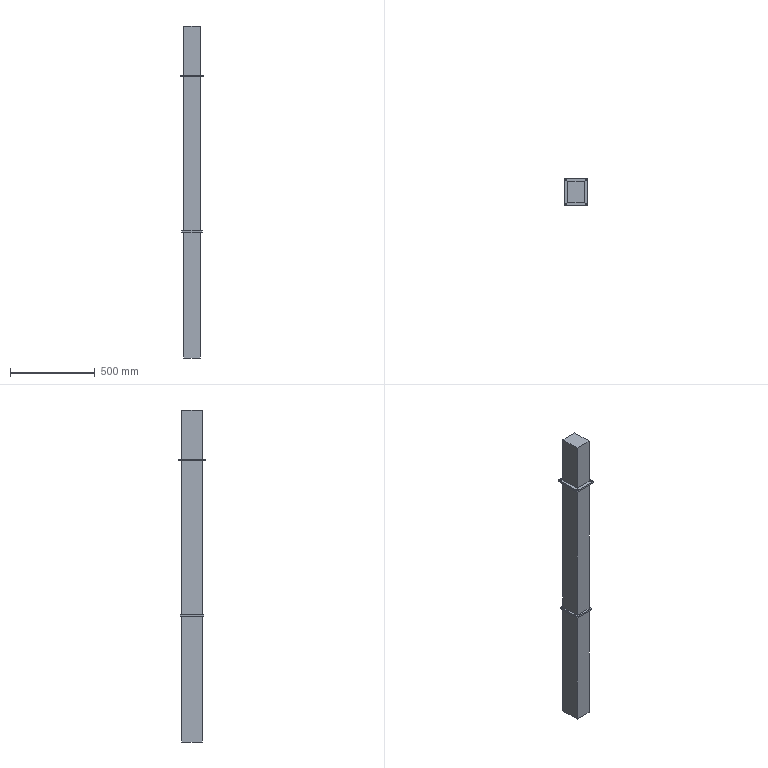Part | SolidWorks | features Cut 2, ICE 2, Extrusion 1 | 1 solid | 34 faces | box 139.912 x 160 x 1959 mm | volume 23636005 mm3 | plane 26 | cylinder 8 | commonest cylinder face diameters 10 x8
STEP:
#1=CARTESIAN_POINT('',(-54.912,230.,400.));
#2=VERTEX_POINT('',#1);
#3=CARTESIAN_POINT('',(-44.912,230.,400.));
#4=VERTEX_POINT('',#3);
#5=CARTESIAN_POINT('',(-49.912,230.,400.));
#6=DIRECTION('',(0.,0.,1.));
#7=DIRECTION('',(1.,0.,0.));
#8=AXIS2_PLACEMENT_3D('',#5,#6,#7);
#9=CIRCLE('',#8,5.);
#10=EDGE_CURVE('',#2,#4,#9,.T.);
#11=ORIENTED_EDGE('',*,*,#10,.F.);
#12=CARTESIAN_POINT('',(-54.912,230.,410.));
#13=VERTEX_POINT('',#12);
#14=CARTESIAN_POINT('',(-54.912,230.,400.));
#15=DIRECTION('',(0.,0.,1.));
#16=VECTOR('',#15,1000.);
#17=LINE('',#14,#16);
#18=EDGE_CURVE('',#2,#13,#17,.T.);
#19=ORIENTED_EDGE('',*,*,#18,.T.);
#20=CARTESIAN_POINT('',(-44.912,230.,410.));
#21=VERTEX_POINT('',#20);
#22=CARTESIAN_POINT('',(-49.912,230.,410.));
#23=DIRECTION('',(0.,0.,1.));
#24=DIRECTION('',(1.,0.,0.));
#25=AXIS2_PLACEMENT_3D('',#22,#23,#24);
#26=CIRCLE('',#25,5.);
#27=EDGE_CURVE('',#13,#21,#26,.T.);
#28=ORIENTED_EDGE('',*,*,#27,.T.);
#29=CARTESIAN_POINT('',(-44.912,230.,400.));
#30=DIRECTION('',(0.,0.,1.));
#31=VECTOR('',#30,1000.);
#32=LINE('',#29,#31);
#33=EDGE_CURVE('',#4,#21,#32,.T.);
#34=ORIENTED_EDGE('',*,*,#33,.F.);
#35=EDGE_LOOP('',(#11,#19,#28,#34));
#36=FACE_OUTER_BOUND('',#35,.T.);
#37=CARTESIAN_POINT('',(-49.912,230.,400.));
#38=DIRECTION('',(0.,0.,1.));
#39=DIRECTION('',(1.,0.,0.));
#40=AXIS2_PLACEMENT_3D('',#37,#38,#39);
#41=CYLINDRICAL_SURFACE('',#40,5.);
#42=ADVANCED_FACE('',(#36),#41,.F.);
#43=CARTESIAN_POINT('',(-54.912,90.,400.));
#44=VERTEX_POINT('',#43);
#45=CARTESIAN_POINT('',(-44.912,90.,400.));
#46=VERTEX_POINT('',#45);
#47=CARTESIAN_POINT('',(-49.912,90.,400.));
#48=DIRECTION('',(0.,0.,1.));
#49=DIRECTION('',(1.,0.,0.));
#50=AXIS2_PLACEMENT_3D('',#47,#48,#49);
#51=CIRCLE('',#50,5.);
#52=EDGE_CURVE('',#44,#46,#51,.T.);
#53=ORIENTED_EDGE('',*,*,#52,.F.);
#54=CARTESIAN_POINT('',(-54.912,90.,410.));
#55=VERTEX_POINT('',#54);
#56=CARTESIAN_POINT('',(-54.912,90.,400.));
#57=DIRECTION('',(0.,0.,1.));
#58=VECTOR('',#57,1000.);
#59=LINE('',#56,#58);
#60=EDGE_CURVE('',#44,#55,#59,.T.);
#61=ORIENTED_EDGE('',*,*,#60,.T.);
#62=CARTESIAN_POINT('',(-44.912,90.,410.));
#63=VERTEX_POINT('',#62);
#64=CARTESIAN_POINT('',(-49.912,90.,410.));
#65=DIRECTION('',(0.,0.,1.));
#66=DIRECTION('',(1.,0.,0.));
#67=AXIS2_PLACEMENT_3D('',#64,#65,#66);
#68=CIRCLE('',#67,5.);
#69=EDGE_CURVE('',#55,#63,#68,.T.);
#70=ORIENTED_EDGE('',*,*,#69,.T.);
#71=CARTESIAN_POINT('',(-44.912,90.,400.));
#72=DIRECTION('',(0.,0.,1.));
#73=VECTOR('',#72,1000.);
#74=LINE('',#71,#73);
#75=EDGE_CURVE('',#46,#63,#74,.T.);
#76=ORIENTED_EDGE('',*,*,#75,.F.);
#77=EDGE_LOOP('',(#53,#61,#70,#76));
#78=FACE_OUTER_BOUND('',#77,.T.);
#79=CARTESIAN_POINT('',(-49.912,90.,400.));
#80=DIRECTION('',(0.,0.,1.));
#81=DIRECTION('',(1.,0.,0.));
#82=AXIS2_PLACEMENT_3D('',#79,#80,#81);
#83=CYLINDRICAL_SURFACE('',#82,5.);
#84=ADVANCED_FACE('',(#78),#83,.F.);
#85=CARTESIAN_POINT('',(65.,90.,400.));
#86=VERTEX_POINT('',#85);
#87=CARTESIAN_POINT('',(75.,90.,400.));
#88=VERTEX_POINT('',#87);
#89=CARTESIAN_POINT('',(70.,90.,400.));
#90=DIRECTION('',(0.,0.,1.));
#91=DIRECTION('',(1.,0.,0.));
#92=AXIS2_PLACEMENT_3D('',#89,#90,#91);
#93=CIRCLE('',#92,5.);
#94=EDGE_CURVE('',#86,#88,#93,.T.);
#95=ORIENTED_EDGE('',*,*,#94,.F.);
#96=CARTESIAN_POINT('',(65.,90.,410.));
#97=VERTEX_POINT('',#96);
#98=CARTESIAN_POINT('',(65.,90.,400.));
#99=DIRECTION('',(0.,0.,1.));
#100=VECTOR('',#99,1000.);
#101=LINE('',#98,#100);
#102=EDGE_CURVE('',#86,#97,#101,.T.);
#103=ORIENTED_EDGE('',*,*,#102,.T.);
#104=CARTESIAN_POINT('',(75.,90.,410.));
#105=VERTEX_POINT('',#104);
#106=CARTESIAN_POINT('',(70.,90.,410.));
#107=DIRECTION('',(0.,0.,1.));
#108=DIRECTION('',(1.,0.,0.));
#109=AXIS2_PLACEMENT_3D('',#106,#107,#108);
#110=CIRCLE('',#109,5.);
#111=EDGE_CURVE('',#97,#105,#110,.T.);
#112=ORIENTED_EDGE('',*,*,#111,.T.);
#113=CARTESIAN_POINT('',(75.,90.,400.));
#114=DIRECTION('',(0.,0.,1.));
#115=VECTOR('',#114,1000.);
#116=LINE('',#113,#115);
#117=EDGE_CURVE('',#88,#105,#116,.T.);
#118=ORIENTED_EDGE('',*,*,#117,.F.);
#119=EDGE_LOOP('',(#95,#103,#112,#118));
#120=FACE_OUTER_BOUND('',#119,.T.);
#121=CARTESIAN_POINT('',(70.,90.,400.));
#122=DIRECTION('',(0.,0.,1.));
#123=DIRECTION('',(1.,0.,0.));
#124=AXIS2_PLACEMENT_3D('',#121,#122,#123);
#125=CYLINDRICAL_SURFACE('',#124,5.);
#126=ADVANCED_FACE('',(#120),#125,.F.);
#127=CARTESIAN_POINT('',(65.,230.,400.));
#128=VERTEX_POINT('',#127);
#129=CARTESIAN_POINT('',(75.,230.,400.));
#130=VERTEX_POINT('',#129);
#131=CARTESIAN_POINT('',(70.,230.,400.));
#132=DIRECTION('',(0.,0.,1.));
#133=DIRECTION('',(1.,0.,0.));
#134=AXIS2_PLACEMENT_3D('',#131,#132,#133);
#135=CIRCLE('',#134,5.);
#136=EDGE_CURVE('',#128,#130,#135,.T.);
#137=ORIENTED_EDGE('',*,*,#136,.F.);
#138=CARTESIAN_POINT('',(65.,230.,410.));
#139=VERTEX_POINT('',#138);
#140=CARTESIAN_POINT('',(65.,230.,400.));
#141=DIRECTION('',(0.,0.,1.));
#142=VECTOR('',#141,1000.);
#143=LINE('',#140,#142);
#144=EDGE_CURVE('',#128,#139,#143,.T.);
#145=ORIENTED_EDGE('',*,*,#144,.T.);
#146=CARTESIAN_POINT('',(75.,230.,410.));
#147=VERTEX_POINT('',#146);
#148=CARTESIAN_POINT('',(70.,230.,410.));
#149=DIRECTION('',(0.,0.,1.));
#150=DIRECTION('',(1.,0.,0.));
#151=AXIS2_PLACEMENT_3D('',#148,#149,#150);
#152=CIRCLE('',#151,5.);
#153=EDGE_CURVE('',#139,#147,#152,.T.);
#154=ORIENTED_EDGE('',*,*,#153,.T.);
#155=CARTESIAN_POINT('',(75.,230.,400.));
#156=DIRECTION('',(0.,0.,1.));
#157=VECTOR('',#156,1000.);
#158=LINE('',#155,#157);
#159=EDGE_CURVE('',#130,#147,#158,.T.);
#160=ORIENTED_EDGE('',*,*,#159,.F.);
#161=EDGE_LOOP('',(#137,#145,#154,#160));
#162=FACE_OUTER_BOUND('',#161,.T.);
#163=CARTESIAN_POINT('',(70.,230.,400.));
#164=DIRECTION('',(0.,0.,1.));
#165=DIRECTION('',(1.,0.,0.));
#166=AXIS2_PLACEMENT_3D('',#163,#164,#165);
#167=CYLINDRICAL_SURFACE('',#166,5.);
#168=ADVANCED_FACE('',(#162),#167,.F.);
#169=CARTESIAN_POINT('',(-39.912,220.,400.));
#170=VERTEX_POINT('',#169);
#171=CARTESIAN_POINT('',(-39.912,100.,400.));
#172=VERTEX_POINT('',#171);
#173=CARTESIAN_POINT('',(-39.912,220.,400.));
#174=DIRECTION('',(0.,-1.,0.));
#175=VECTOR('',#174,1000.);
#176=LINE('',#173,#175);
#177=EDGE_CURVE('',#170,#172,#176,.T.);
#178=ORIENTED_EDGE('',*,*,#177,.F.);
#179=CARTESIAN_POINT('',(-39.912,220.,-509.));
#180=VERTEX_POINT('',#179);
#181=CARTESIAN_POINT('',(-39.912,220.,-2285.));
#182=DIRECTION('',(0.,0.,1.));
#183=VECTOR('',#182,1000.);
#184=LINE('',#181,#183);
#185=EDGE_CURVE('',#180,#170,#184,.T.);
#186=ORIENTED_EDGE('',*,*,#185,.F.);
#187=CARTESIAN_POINT('',(-39.912,100.,-509.));
#188=VERTEX_POINT('',#187);
#189=CARTESIAN_POINT('',(-39.912,100.,-509.));
#190=DIRECTION('',(0.,1.,0.));
#191=VECTOR('',#190,1000.);
#192=LINE('',#189,#191);
#193=EDGE_CURVE('',#188,#180,#192,.T.);
#194=ORIENTED_EDGE('',*,*,#193,.F.);
#195=CARTESIAN_POINT('',(-39.912,100.,-2285.));
#196=DIRECTION('',(0.,0.,1.));
#197=VECTOR('',#196,1000.);
#198=LINE('',#195,#197);
#199=EDGE_CURVE('',#188,#172,#198,.T.);
#200=ORIENTED_EDGE('',*,*,#199,.T.);
#201=EDGE_LOOP('',(#178,#186,#194,#200));
#202=FACE_OUTER_BOUND('',#201,.T.);
#203=CARTESIAN_POINT('',(-39.912,220.,-2285.));
#204=DIRECTION('',(1.,0.,0.));
#205=DIRECTION('',(0.,0.,-1.));
#206=AXIS2_PLACEMENT_3D('',#203,#204,#205);
#207=PLANE('',#206);
#208=ADVANCED_FACE('',(#202),#207,.F.);
#209=ORIENTED_EDGE('',*,*,#185,.T.);
#210=CARTESIAN_POINT('',(60.,220.,400.));
#211=VERTEX_POINT('',#210);
#212=CARTESIAN_POINT('',(-60.,220.,400.));
#213=DIRECTION('',(1.,0.,0.));
#214=VECTOR('',#213,1000.);
#215=LINE('',#212,#214);
#216=EDGE_CURVE('',#170,#211,#215,.T.);
#217=ORIENTED_EDGE('',*,*,#216,.T.);
#218=CARTESIAN_POINT('',(60.,220.,-509.));
#219=VERTEX_POINT('',#218);
#220=CARTESIAN_POINT('',(60.,220.,-1259.));
#221=DIRECTION('',(0.,0.,1.));
#222=VECTOR('',#221,1000.);
#223=LINE('',#220,#222);
#224=EDGE_CURVE('',#219,#211,#223,.T.);
#225=ORIENTED_EDGE('',*,*,#224,.F.);
#226=CARTESIAN_POINT('',(-39.912,220.,-509.));
#227=DIRECTION('',(1.,0.,0.));
#228=VECTOR('',#227,1000.);
#229=LINE('',#226,#228);
#230=EDGE_CURVE('',#180,#219,#229,.T.);
#231=ORIENTED_EDGE('',*,*,#230,.F.);
#232=EDGE_LOOP('',(#209,#217,#225,#231));
#233=FACE_OUTER_BOUND('',#232,.T.);
#234=CARTESIAN_POINT('',(-60.,220.,-1259.));
#235=DIRECTION('',(0.,1.,0.));
#236=DIRECTION('',(0.,0.,1.));
#237=AXIS2_PLACEMENT_3D('',#234,#235,#236);
#238=PLANE('',#237);
#239=ADVANCED_FACE('',(#233),#238,.T.);
#240=CARTESIAN_POINT('',(60.,100.,-509.));
#241=VERTEX_POINT('',#240);
#242=CARTESIAN_POINT('',(60.,100.,400.));
#243=VERTEX_POINT('',#242);
#244=CARTESIAN_POINT('',(60.,100.,-1259.));
#245=DIRECTION('',(0.,0.,1.));
#246=VECTOR('',#245,1000.);
#247=LINE('',#244,#246);
#248=EDGE_CURVE('',#241,#243,#247,.T.);
#249=ORIENTED_EDGE('',*,*,#248,.T.);
#250=CARTESIAN_POINT('',(-60.,100.,400.));
#251=DIRECTION('',(-1.,0.,0.));
#252=VECTOR('',#251,1000.);
#253=LINE('',#250,#252);
#254=EDGE_CURVE('',#243,#172,#253,.T.);
#255=ORIENTED_EDGE('',*,*,#254,.T.);
#256=ORIENTED_EDGE('',*,*,#199,.F.);
#257=CARTESIAN_POINT('',(-39.912,100.,-509.));
#258=DIRECTION('',(-1.,0.,0.));
#259=VECTOR('',#258,1000.);
#260=LINE('',#257,#259);
#261=EDGE_CURVE('',#241,#188,#260,.T.);
#262=ORIENTED_EDGE('',*,*,#261,.F.);
#263=EDGE_LOOP('',(#249,#255,#256,#262));
#264=FACE_OUTER_BOUND('',#263,.T.);
#265=CARTESIAN_POINT('',(-60.,100.,-1259.));
#266=DIRECTION('',(0.,-1.,0.));
#267=DIRECTION('',(0.,0.,-1.));
#268=AXIS2_PLACEMENT_3D('',#265,#266,#267);
#269=PLANE('',#268);
#270=ADVANCED_FACE('',(#264),#269,.T.);
#271=ORIENTED_EDGE('',*,*,#224,.T.);
#272=CARTESIAN_POINT('',(60.,220.,400.));
#273=DIRECTION('',(0.,-1.,0.));
#274=VECTOR('',#273,1000.);
#275=LINE('',#272,#274);
#276=EDGE_CURVE('',#211,#243,#275,.T.);
#277=ORIENTED_EDGE('',*,*,#276,.T.);
#278=ORIENTED_EDGE('',*,*,#248,.F.);
#279=CARTESIAN_POINT('',(60.,100.,-509.));
#280=DIRECTION('',(0.,-1.,0.));
#281=VECTOR('',#280,1000.);
#282=LINE('',#279,#281);
#283=EDGE_CURVE('',#219,#241,#282,.T.);
#284=ORIENTED_EDGE('',*,*,#283,.F.);
#285=EDGE_LOOP('',(#271,#277,#278,#284));
#286=FACE_OUTER_BOUND('',#285,.T.);
#287=CARTESIAN_POINT('',(60.,220.,-1259.));
#288=DIRECTION('',(1.,0.,0.));
#289=DIRECTION('',(0.,1.,0.));
#290=AXIS2_PLACEMENT_3D('',#287,#288,#289);
#291=PLANE('',#290);
#292=ADVANCED_FACE('',(#286),#291,.T.);
#293=CARTESIAN_POINT('',(60.,220.,-1259.));
#294=VERTEX_POINT('',#293);
#295=CARTESIAN_POINT('',(60.,220.,-519.));
#296=VERTEX_POINT('',#295);
#297=CARTESIAN_POINT('',(60.,220.,-1259.));
#298=DIRECTION('',(0.,0.,1.));
#299=VECTOR('',#298,1000.);
#300=LINE('',#297,#299);
#301=EDGE_CURVE('',#294,#296,#300,.T.);
#302=ORIENTED_EDGE('',*,*,#301,.T.);
#303=CARTESIAN_POINT('',(60.,100.,-519.));
#304=VERTEX_POINT('',#303);
#305=CARTESIAN_POINT('',(60.,100.,-519.));
#306=DIRECTION('',(0.,-1.,0.));
#307=VECTOR('',#306,1000.);
#308=LINE('',#305,#307);
#309=EDGE_CURVE('',#296,#304,#308,.T.);
#310=ORIENTED_EDGE('',*,*,#309,.T.);
#311=CARTESIAN_POINT('',(60.,100.,-1259.));
#312=VERTEX_POINT('',#311);
#313=CARTESIAN_POINT('',(60.,100.,-1259.));
#314=DIRECTION('',(0.,0.,1.));
#315=VECTOR('',#314,1000.);
#316=LINE('',#313,#315);
#317=EDGE_CURVE('',#312,#304,#316,.T.);
#318=ORIENTED_EDGE('',*,*,#317,.F.);
#319=CARTESIAN_POINT('',(60.,220.,-1259.));
#320=DIRECTION('',(0.,1.,0.));
#321=VECTOR('',#320,1000.);
#322=LINE('',#319,#321);
#323=EDGE_CURVE('',#312,#294,#322,.T.);
#324=ORIENTED_EDGE('',*,*,#323,.T.);
#325=EDGE_LOOP('',(#302,#310,#318,#324));
#326=FACE_OUTER_BOUND('',#325,.T.);
#327=CARTESIAN_POINT('',(60.,220.,-1259.));
#328=DIRECTION('',(1.,0.,0.));
#329=DIRECTION('',(0.,1.,0.));
#330=AXIS2_PLACEMENT_3D('',#327,#328,#329);
#331=PLANE('',#330);
#332=ADVANCED_FACE('',(#326),#331,.T.);
#333=ORIENTED_EDGE('',*,*,#317,.T.);
#334=CARTESIAN_POINT('',(-39.912,100.,-519.));
#335=VERTEX_POINT('',#334);
#336=CARTESIAN_POINT('',(-39.912,100.,-519.));
#337=DIRECTION('',(-1.,0.,0.));
#338=VECTOR('',#337,1000.);
#339=LINE('',#336,#338);
#340=EDGE_CURVE('',#304,#335,#339,.T.);
#341=ORIENTED_EDGE('',*,*,#340,.T.);
#342=CARTESIAN_POINT('',(-39.912,100.,-1259.));
#343=VERTEX_POINT('',#342);
#344=CARTESIAN_POINT('',(-39.912,100.,-2285.));
#345=DIRECTION('',(0.,0.,1.));
#346=VECTOR('',#345,1000.);
#347=LINE('',#344,#346);
#348=EDGE_CURVE('',#343,#335,#347,.T.);
#349=ORIENTED_EDGE('',*,*,#348,.F.);
#350=CARTESIAN_POINT('',(-60.,100.,-1259.));
#351=DIRECTION('',(1.,0.,0.));
#352=VECTOR('',#351,1000.);
#353=LINE('',#350,#352);
#354=EDGE_CURVE('',#343,#312,#353,.T.);
#355=ORIENTED_EDGE('',*,*,#354,.T.);
#356=EDGE_LOOP('',(#333,#341,#349,#355));
#357=FACE_OUTER_BOUND('',#356,.T.);
#358=CARTESIAN_POINT('',(-60.,100.,-1259.));
#359=DIRECTION('',(0.,-1.,0.));
#360=DIRECTION('',(0.,0.,-1.));
#361=AXIS2_PLACEMENT_3D('',#358,#359,#360);
#362=PLANE('',#361);
#363=ADVANCED_FACE('',(#357),#362,.T.);
#364=CARTESIAN_POINT('',(-39.912,220.,-1259.));
#365=VERTEX_POINT('',#364);
#366=CARTESIAN_POINT('',(-39.912,220.,-519.));
#367=VERTEX_POINT('',#366);
#368=CARTESIAN_POINT('',(-39.912,220.,-2285.));
#369=DIRECTION('',(0.,0.,1.));
#370=VECTOR('',#369,1000.);
#371=LINE('',#368,#370);
#372=EDGE_CURVE('',#365,#367,#371,.T.);
#373=ORIENTED_EDGE('',*,*,#372,.T.);
#374=CARTESIAN_POINT('',(-39.912,220.,-519.));
#375=DIRECTION('',(1.,0.,0.));
#376=VECTOR('',#375,1000.);
#377=LINE('',#374,#376);
#378=EDGE_CURVE('',#367,#296,#377,.T.);
#379=ORIENTED_EDGE('',*,*,#378,.T.);
#380=ORIENTED_EDGE('',*,*,#301,.F.);
#381=CARTESIAN_POINT('',(-60.,220.,-1259.));
#382=DIRECTION('',(-1.,0.,0.));
#383=VECTOR('',#382,1000.);
#384=LINE('',#381,#383);
#385=EDGE_CURVE('',#294,#365,#384,.T.);
#386=ORIENTED_EDGE('',*,*,#385,.T.);
#387=EDGE_LOOP('',(#373,#379,#380,#386));
#388=FACE_OUTER_BOUND('',#387,.T.);
#389=CARTESIAN_POINT('',(-60.,220.,-1259.));
#390=DIRECTION('',(0.,1.,0.));
#391=DIRECTION('',(0.,0.,1.));
#392=AXIS2_PLACEMENT_3D('',#389,#390,#391);
#393=PLANE('',#392);
#394=ADVANCED_FACE('',(#388),#393,.T.);
#395=CARTESIAN_POINT('',(-39.912,100.,-519.));
#396=DIRECTION('',(0.,1.,0.));
#397=VECTOR('',#396,1000.);
#398=LINE('',#395,#397);
#399=EDGE_CURVE('',#335,#367,#398,.T.);
#400=ORIENTED_EDGE('',*,*,#399,.T.);
#401=ORIENTED_EDGE('',*,*,#372,.F.);
#402=CARTESIAN_POINT('',(-39.912,0.,-1259.));
#403=DIRECTION('',(0.,1.,0.));
#404=VECTOR('',#403,1000.);
#405=LINE('',#402,#404);
#406=EDGE_CURVE('',#343,#365,#405,.T.);
#407=ORIENTED_EDGE('',*,*,#406,.F.);
#408=ORIENTED_EDGE('',*,*,#348,.T.);
#409=EDGE_LOOP('',(#400,#401,#407,#408));
#410=FACE_OUTER_BOUND('',#409,.T.);
#411=CARTESIAN_POINT('',(-39.912,220.,-2285.));
#412=DIRECTION('',(1.,0.,0.));
#413=DIRECTION('',(0.,0.,-1.));
#414=AXIS2_PLACEMENT_3D('',#411,#412,#413);
#415=PLANE('',#414);
#416=ADVANCED_FACE('',(#410),#415,.F.);
#417=ORIENTED_EDGE('',*,*,#354,.F.);
#418=ORIENTED_EDGE('',*,*,#406,.T.);
#419=ORIENTED_EDGE('',*,*,#385,.F.);
#420=ORIENTED_EDGE('',*,*,#323,.F.);
#421=EDGE_LOOP('',(#417,#418,#419,#420));
#422=FACE_OUTER_BOUND('',#421,.T.);
#423=CARTESIAN_POINT('',(0.,0.,-1259.));
#424=DIRECTION('',(0.,0.,1.));
#425=DIRECTION('',(1.,0.,0.));
#426=AXIS2_PLACEMENT_3D('',#423,#424,#425);
#427=PLANE('',#426);
#428=ADVANCED_FACE('',(#422),#427,.F.);
#429=CARTESIAN_POINT('',(70.,90.,-519.));
#430=VERTEX_POINT('',#429);
#431=CARTESIAN_POINT('',(-49.912,90.,-519.));
#432=VERTEX_POINT('',#431);
#433=CARTESIAN_POINT('',(-49.912,90.,-519.));
#434=DIRECTION('',(-1.,0.,0.));
#435=VECTOR('',#434,1000.);
#436=LINE('',#433,#435);
#437=EDGE_CURVE('',#430,#432,#436,.T.);
#438=ORIENTED_EDGE('',*,*,#437,.T.);
#439=CARTESIAN_POINT('',(-49.912,230.,-519.));
#440=VERTEX_POINT('',#439);
#441=CARTESIAN_POINT('',(-49.912,90.,-519.));
#442=DIRECTION('',(0.,1.,0.));
#443=VECTOR('',#442,1000.);
#444=LINE('',#441,#443);
#445=EDGE_CURVE('',#432,#440,#444,.T.);
#446=ORIENTED_EDGE('',*,*,#445,.T.);
#447=CARTESIAN_POINT('',(70.,230.,-519.));
#448=VERTEX_POINT('',#447);
#449=CARTESIAN_POINT('',(-49.912,230.,-519.));
#450=DIRECTION('',(1.,0.,0.));
#451=VECTOR('',#450,1000.);
#452=LINE('',#449,#451);
#453=EDGE_CURVE('',#440,#448,#452,.T.);
#454=ORIENTED_EDGE('',*,*,#453,.T.);
#455=CARTESIAN_POINT('',(70.,90.,-519.));
#456=DIRECTION('',(0.,-1.,0.));
#457=VECTOR('',#456,1000.);
#458=LINE('',#455,#457);
#459=EDGE_CURVE('',#448,#430,#458,.T.);
#460=ORIENTED_EDGE('',*,*,#459,.T.);
#461=EDGE_LOOP('',(#438,#446,#454,#460));
#462=FACE_OUTER_BOUND('',#461,.T.);
#463=ORIENTED_EDGE('',*,*,#399,.F.);
#464=ORIENTED_EDGE('',*,*,#340,.F.);
#465=ORIENTED_EDGE('',*,*,#309,.F.);
#466=ORIENTED_EDGE('',*,*,#378,.F.);
#467=EDGE_LOOP('',(#463,#464,#465,#466));
#468=FACE_BOUND('',#467,.T.);
#469=CARTESIAN_POINT('',(0.,0.,-519.));
#470=DIRECTION('',(0.,0.,1.));
#471=DIRECTION('',(1.,0.,0.));
#472=AXIS2_PLACEMENT_3D('',#469,#470,#471);
#473=PLANE('',#472);
#474=ADVANCED_FACE('',(#462,#468),#473,.F.);
#475=CARTESIAN_POINT('',(70.,90.,-509.));
#476=VERTEX_POINT('',#475);
#477=CARTESIAN_POINT('',(-49.912,90.,-509.));
#478=VERTEX_POINT('',#477);
#479=CARTESIAN_POINT('',(-49.912,90.,-509.));
#480=DIRECTION('',(-1.,0.,0.));
#481=VECTOR('',#480,1000.);
#482=LINE('',#479,#481);
#483=EDGE_CURVE('',#476,#478,#482,.T.);
#484=ORIENTED_EDGE('',*,*,#483,.F.);
#485=CARTESIAN_POINT('',(70.,230.,-509.));
#486=VERTEX_POINT('',#485);
#487=CARTESIAN_POINT('',(70.,90.,-509.));
#488=DIRECTION('',(0.,-1.,0.));
#489=VECTOR('',#488,1000.);
#490=LINE('',#487,#489);
#491=EDGE_CURVE('',#486,#476,#490,.T.);
#492=ORIENTED_EDGE('',*,*,#491,.F.);
#493=CARTESIAN_POINT('',(-49.912,230.,-509.));
#494=VERTEX_POINT('',#493);
#495=CARTESIAN_POINT('',(-49.912,230.,-509.));
#496=DIRECTION('',(1.,0.,0.));
#497=VECTOR('',#496,1000.);
#498=LINE('',#495,#497);
#499=EDGE_CURVE('',#494,#486,#498,.T.);
#500=ORIENTED_EDGE('',*,*,#499,.F.);
#501=CARTESIAN_POINT('',(-49.912,90.,-509.));
#502=DIRECTION('',(0.,1.,0.));
#503=VECTOR('',#502,1000.);
#504=LINE('',#501,#503);
#505=EDGE_CURVE('',#478,#494,#504,.T.);
#506=ORIENTED_EDGE('',*,*,#505,.F.);
#507=EDGE_LOOP('',(#484,#492,#500,#506));
#508=FACE_OUTER_BOUND('',#507,.T.);
#509=ORIENTED_EDGE('',*,*,#261,.T.);
#510=ORIENTED_EDGE('',*,*,#193,.T.);
#511=ORIENTED_EDGE('',*,*,#230,.T.);
#512=ORIENTED_EDGE('',*,*,#283,.T.);
#513=EDGE_LOOP('',(#509,#510,#511,#512));
#514=FACE_BOUND('',#513,.T.);
#515=CARTESIAN_POINT('',(0.,0.,-509.));
#516=DIRECTION('',(0.,0.,1.));
#517=DIRECTION('',(1.,0.,0.));
#518=AXIS2_PLACEMENT_3D('',#515,#516,#517);
#519=PLANE('',#518);
#520=ADVANCED_FACE('',(#508,#514),#519,.T.);
#521=ORIENTED_EDGE('',*,*,#483,.T.);
#522=CARTESIAN_POINT('',(-49.912,90.,-519.));
#523=DIRECTION('',(0.,0.,1.));
#524=VECTOR('',#523,1000.);
#525=LINE('',#522,#524);
#526=EDGE_CURVE('',#432,#478,#525,.T.);
#527=ORIENTED_EDGE('',*,*,#526,.F.);
#528=ORIENTED_EDGE('',*,*,#437,.F.);
#529=CARTESIAN_POINT('',(70.,90.,-519.));
#530=DIRECTION('',(0.,0.,1.));
#531=VECTOR('',#530,1000.);
#532=LINE('',#529,#531);
#533=EDGE_CURVE('',#430,#476,#532,.T.);
#534=ORIENTED_EDGE('',*,*,#533,.T.);
#535=EDGE_LOOP('',(#521,#527,#528,#534));
#536=FACE_OUTER_BOUND('',#535,.T.);
#537=CARTESIAN_POINT('',(-49.912,90.,-519.));
#538=DIRECTION('',(0.,1.,0.));
#539=DIRECTION('',(0.,0.,1.));
#540=AXIS2_PLACEMENT_3D('',#537,#538,#539);
#541=PLANE('',#540);
#542=ADVANCED_FACE('',(#536),#541,.F.);
#543=ORIENTED_EDGE('',*,*,#505,.T.);
#544=CARTESIAN_POINT('',(-49.912,230.,-519.));
#545=DIRECTION('',(0.,0.,1.));
#546=VECTOR('',#545,1000.);
#547=LINE('',#544,#546);
#548=EDGE_CURVE('',#440,#494,#547,.T.);
#549=ORIENTED_EDGE('',*,*,#548,.F.);
#550=ORIENTED_EDGE('',*,*,#445,.F.);
#551=ORIENTED_EDGE('',*,*,#526,.T.);
#552=EDGE_LOOP('',(#543,#549,#550,#551));
#553=FACE_OUTER_BOUND('',#552,.T.);
#554=CARTESIAN_POINT('',(-49.912,90.,-519.));
#555=DIRECTION('',(1.,0.,0.));
#556=DIRECTION('',(0.,0.,-1.));
#557=AXIS2_PLACEMENT_3D('',#554,#555,#556);
#558=PLANE('',#557);
#559=ADVANCED_FACE('',(#553),#558,.F.);
#560=ORIENTED_EDGE('',*,*,#499,.T.);
#561=CARTESIAN_POINT('',(70.,230.,-519.));
#562=DIRECTION('',(0.,0.,1.));
#563=VECTOR('',#562,1000.);
#564=LINE('',#561,#563);
#565=EDGE_CURVE('',#448,#486,#564,.T.);
#566=ORIENTED_EDGE('',*,*,#565,.F.);
#567=ORIENTED_EDGE('',*,*,#453,.F.);
#568=ORIENTED_EDGE('',*,*,#548,.T.);
#569=EDGE_LOOP('',(#560,#566,#567,#568));
#570=FACE_OUTER_BOUND('',#569,.T.);
#571=CARTESIAN_POINT('',(-49.912,230.,-519.));
#572=DIRECTION('',(0.,-1.,0.));
#573=DIRECTION('',(0.,0.,-1.));
#574=AXIS2_PLACEMENT_3D('',#571,#572,#573);
#575=PLANE('',#574);
#576=ADVANCED_FACE('',(#570),#575,.F.);
#577=ORIENTED_EDGE('',*,*,#491,.T.);
#578=ORIENTED_EDGE('',*,*,#533,.F.);
#579=ORIENTED_EDGE('',*,*,#459,.F.);
#580=ORIENTED_EDGE('',*,*,#565,.T.);
#581=EDGE_LOOP('',(#577,#578,#579,#580));
#582=FACE_OUTER_BOUND('',#581,.T.);
#583=CARTESIAN_POINT('',(70.,90.,-519.));
#584=DIRECTION('',(-1.,0.,0.));
#585=DIRECTION('',(0.,0.,1.));
#586=AXIS2_PLACEMENT_3D('',#583,#584,#585);
#587=PLANE('',#586);
#588=ADVANCED_FACE('',(#582),#587,.F.);
#589=CARTESIAN_POINT('',(-49.912,230.,410.));
#590=DIRECTION('',(0.,0.,1.));
#591=DIRECTION('',(1.,0.,0.));
#592=AXIS2_PLACEMENT_3D('',#589,#590,#591);
#593=CIRCLE('',#592,5.);
#594=EDGE_CURVE('',#21,#13,#593,.T.);
#595=ORIENTED_EDGE('',*,*,#594,.F.);
#596=ORIENTED_EDGE('',*,*,#27,.F.);
#597=EDGE_LOOP('',(#595,#596));
#598=FACE_BOUND('',#597,.T.);
#599=CARTESIAN_POINT('',(-49.912,90.,410.));
#600=DIRECTION('',(0.,0.,1.));
#601=DIRECTION('',(1.,0.,0.));
#602=AXIS2_PLACEMENT_3D('',#599,#600,#601);
#603=CIRCLE('',#602,5.);
#604=EDGE_CURVE('',#63,#55,#603,.T.);
#605=ORIENTED_EDGE('',*,*,#604,.F.);
#606=ORIENTED_EDGE('',*,*,#69,.F.);
#607=EDGE_LOOP('',(#605,#606));
#608=FACE_BOUND('',#607,.T.);
#609=CARTESIAN_POINT('',(70.,90.,410.));
#610=DIRECTION('',(0.,0.,1.));
#611=DIRECTION('',(1.,0.,0.));
#612=AXIS2_PLACEMENT_3D('',#609,#610,#611);
#613=CIRCLE('',#612,5.);
#614=EDGE_CURVE('',#105,#97,#613,.T.);
#615=ORIENTED_EDGE('',*,*,#614,.F.);
#616=ORIENTED_EDGE('',*,*,#111,.F.);
#617=EDGE_LOOP('',(#615,#616));
#618=FACE_BOUND('',#617,.T.);
#619=CARTESIAN_POINT('',(70.,230.,410.));
#620=DIRECTION('',(0.,0.,1.));
#621=DIRECTION('',(1.,0.,0.));
#622=AXIS2_PLACEMENT_3D('',#619,#620,#621);
#623=CIRCLE('',#622,5.);
#624=EDGE_CURVE('',#147,#139,#623,.T.);
#625=ORIENTED_EDGE('',*,*,#624,.F.);
#626=ORIENTED_EDGE('',*,*,#153,.F.);
#627=EDGE_LOOP('',(#625,#626));
#628=FACE_BOUND('',#627,.T.);
#629=CARTESIAN_POINT('',(80.,240.,410.));
#630=VERTEX_POINT('',#629);
#631=CARTESIAN_POINT('',(-59.912,240.,410.));
#632=VERTEX_POINT('',#631);
#633=CARTESIAN_POINT('',(80.,240.,410.));
#634=DIRECTION('',(-1.,0.,0.));
#635=VECTOR('',#634,1000.);
#636=LINE('',#633,#635);
#637=EDGE_CURVE('',#630,#632,#636,.T.);
#638=ORIENTED_EDGE('',*,*,#637,.T.);
#639=CARTESIAN_POINT('',(-59.912,80.,410.));
#640=VERTEX_POINT('',#639);
#641=CARTESIAN_POINT('',(-59.912,240.,410.));
#642=DIRECTION('',(0.,-1.,0.));
#643=VECTOR('',#642,1000.);
#644=LINE('',#641,#643);
#645=EDGE_CURVE('',#632,#640,#644,.T.);
#646=ORIENTED_EDGE('',*,*,#645,.T.);
#647=CARTESIAN_POINT('',(80.,80.,410.));
#648=VERTEX_POINT('',#647);
#649=CARTESIAN_POINT('',(-59.912,80.,410.));
#650=DIRECTION('',(1.,0.,0.));
#651=VECTOR('',#650,1000.);
#652=LINE('',#649,#651);
#653=EDGE_CURVE('',#640,#648,#652,.T.);
#654=ORIENTED_EDGE('',*,*,#653,.T.);
#655=CARTESIAN_POINT('',(80.,80.,410.));
#656=DIRECTION('',(0.,1.,0.));
#657=VECTOR('',#656,1000.);
#658=LINE('',#655,#657);
#659=EDGE_CURVE('',#648,#630,#658,.T.);
#660=ORIENTED_EDGE('',*,*,#659,.T.);
#661=EDGE_LOOP('',(#638,#646,#654,#660));
#662=FACE_OUTER_BOUND('',#661,.T.);
#663=CARTESIAN_POINT('',(-39.912,220.,410.));
#664=VERTEX_POINT('',#663);
#665=CARTESIAN_POINT('',(-39.912,100.,410.));
#666=VERTEX_POINT('',#665);
#667=CARTESIAN_POINT('',(-39.912,220.,410.));
#668=DIRECTION('',(0.,-1.,0.));
#669=VECTOR('',#668,1000.);
#670=LINE('',#667,#669);
#671=EDGE_CURVE('',#664,#666,#670,.T.);
#672=ORIENTED_EDGE('',*,*,#671,.F.);
#673=CARTESIAN_POINT('',(60.,220.,410.));
#674=VERTEX_POINT('',#673);
#675=CARTESIAN_POINT('',(-60.,220.,410.));
#676=DIRECTION('',(1.,0.,0.));
#677=VECTOR('',#676,1000.);
#678=LINE('',#675,#677);
#679=EDGE_CURVE('',#664,#674,#678,.T.);
#680=ORIENTED_EDGE('',*,*,#679,.T.);
#681=CARTESIAN_POINT('',(60.,100.,410.));
#682=VERTEX_POINT('',#681);
#683=CARTESIAN_POINT('',(60.,220.,410.));
#684=DIRECTION('',(0.,-1.,0.));
#685=VECTOR('',#684,1000.);
#686=LINE('',#683,#685);
#687=EDGE_CURVE('',#674,#682,#686,.T.);
#688=ORIENTED_EDGE('',*,*,#687,.T.);
#689=CARTESIAN_POINT('',(-60.,100.,410.));
#690=DIRECTION('',(-1.,0.,0.));
#691=VECTOR('',#690,1000.);
#692=LINE('',#689,#691);
#693=EDGE_CURVE('',#682,#666,#692,.T.);
#694=ORIENTED_EDGE('',*,*,#693,.T.);
#695=EDGE_LOOP('',(#672,#680,#688,#694));
#696=FACE_BOUND('',#695,.T.);
#697=CARTESIAN_POINT('',(0.,0.,410.));
#698=DIRECTION('',(0.,0.,1.));
#699=DIRECTION('',(1.,0.,0.));
#700=AXIS2_PLACEMENT_3D('',#697,#698,#699);
#701=PLANE('',#700);
#702=ADVANCED_FACE('',(#598,#608,#618,#628,#662,#696),#701,.T.);
#703=CARTESIAN_POINT('',(-49.912,230.,400.));
#704=DIRECTION('',(0.,0.,1.));
#705=DIRECTION('',(1.,0.,0.));
#706=AXIS2_PLACEMENT_3D('',#703,#704,#705);
#707=CIRCLE('',#706,5.);
#708=EDGE_CURVE('',#4,#2,#707,.T.);
#709=ORIENTED_EDGE('',*,*,#708,.T.);
#710=ORIENTED_EDGE('',*,*,#10,.T.);
#711=EDGE_LOOP('',(#709,#710));
#712=FACE_BOUND('',#711,.T.);
#713=CARTESIAN_POINT('',(-49.912,90.,400.));
#714=DIRECTION('',(0.,0.,1.));
#715=DIRECTION('',(1.,0.,0.));
#716=AXIS2_PLACEMENT_3D('',#713,#714,#715);
#717=CIRCLE('',#716,5.);
#718=EDGE_CURVE('',#46,#44,#717,.T.);
#719=ORIENTED_EDGE('',*,*,#718,.T.);
#720=ORIENTED_EDGE('',*,*,#52,.T.);
#721=EDGE_LOOP('',(#719,#720));
#722=FACE_BOUND('',#721,.T.);
#723=CARTESIAN_POINT('',(70.,90.,400.));
#724=DIRECTION('',(0.,0.,1.));
#725=DIRECTION('',(1.,0.,0.));
#726=AXIS2_PLACEMENT_3D('',#723,#724,#725);
#727=CIRCLE('',#726,5.);
#728=EDGE_CURVE('',#88,#86,#727,.T.);
#729=ORIENTED_EDGE('',*,*,#728,.T.);
#730=ORIENTED_EDGE('',*,*,#94,.T.);
#731=EDGE_LOOP('',(#729,#730));
#732=FACE_BOUND('',#731,.T.);
#733=CARTESIAN_POINT('',(70.,230.,400.));
#734=DIRECTION('',(0.,0.,1.));
#735=DIRECTION('',(1.,0.,0.));
#736=AXIS2_PLACEMENT_3D('',#733,#734,#735);
#737=CIRCLE('',#736,5.);
#738=EDGE_CURVE('',#130,#128,#737,.T.);
#739=ORIENTED_EDGE('',*,*,#738,.T.);
#740=ORIENTED_EDGE('',*,*,#136,.T.);
#741=EDGE_LOOP('',(#739,#740));
#742=FACE_BOUND('',#741,.T.);
#743=CARTESIAN_POINT('',(80.,240.,400.));
#744=VERTEX_POINT('',#743);
#745=CARTESIAN_POINT('',(-59.912,240.,400.));
#746=VERTEX_POINT('',#745);
#747=CARTESIAN_POINT('',(80.,240.,400.));
#748=DIRECTION('',(-1.,0.,0.));
#749=VECTOR('',#748,1000.);
#750=LINE('',#747,#749);
#751=EDGE_CURVE('',#744,#746,#750,.T.);
#752=ORIENTED_EDGE('',*,*,#751,.F.);
#753=CARTESIAN_POINT('',(80.,80.,400.));
#754=VERTEX_POINT('',#753);
#755=CARTESIAN_POINT('',(80.,80.,400.));
#756=DIRECTION('',(0.,1.,0.));
#757=VECTOR('',#756,1000.);
#758=LINE('',#755,#757);
#759=EDGE_CURVE('',#754,#744,#758,.T.);
#760=ORIENTED_EDGE('',*,*,#759,.F.);
#761=CARTESIAN_POINT('',(-59.912,80.,400.));
#762=VERTEX_POINT('',#761);
#763=CARTESIAN_POINT('',(-59.912,80.,400.));
#764=DIRECTION('',(1.,0.,0.));
#765=VECTOR('',#764,1000.);
#766=LINE('',#763,#765);
#767=EDGE_CURVE('',#762,#754,#766,.T.);
#768=ORIENTED_EDGE('',*,*,#767,.F.);
#769=CARTESIAN_POINT('',(-59.912,240.,400.));
#770=DIRECTION('',(0.,-1.,0.));
#771=VECTOR('',#770,1000.);
#772=LINE('',#769,#771);
#773=EDGE_CURVE('',#746,#762,#772,.T.);
#774=ORIENTED_EDGE('',*,*,#773,.F.);
#775=EDGE_LOOP('',(#752,#760,#768,#774));
#776=FACE_OUTER_BOUND('',#775,.T.);
#777=ORIENTED_EDGE('',*,*,#216,.F.);
#778=ORIENTED_EDGE('',*,*,#177,.T.);
#779=ORIENTED_EDGE('',*,*,#254,.F.);
#780=ORIENTED_EDGE('',*,*,#276,.F.);
#781=EDGE_LOOP('',(#777,#778,#779,#780));
#782=FACE_BOUND('',#781,.T.);
#783=CARTESIAN_POINT('',(0.,0.,400.));
#784=DIRECTION('',(0.,0.,1.));
#785=DIRECTION('',(1.,0.,0.));
#786=AXIS2_PLACEMENT_3D('',#783,#784,#785);
#787=PLANE('',#786);
#788=ADVANCED_FACE('',(#712,#722,#732,#742,#776,#782),#787,.F.);
#789=ORIENTED_EDGE('',*,*,#751,.T.);
#790=CARTESIAN_POINT('',(-59.912,240.,410.));
#791=DIRECTION('',(0.,0.,-1.));
#792=VECTOR('',#791,1000.);
#793=LINE('',#790,#792);
#794=EDGE_CURVE('',#632,#746,#793,.T.);
#795=ORIENTED_EDGE('',*,*,#794,.F.);
#796=ORIENTED_EDGE('',*,*,#637,.F.);
#797=CARTESIAN_POINT('',(80.,240.,410.));
#798=DIRECTION('',(0.,0.,-1.));
#799=VECTOR('',#798,1000.);
#800=LINE('',#797,#799);
#801=EDGE_CURVE('',#630,#744,#800,.T.);
#802=ORIENTED_EDGE('',*,*,#801,.T.);
#803=EDGE_LOOP('',(#789,#795,#796,#802));
#804=FACE_OUTER_BOUND('',#803,.T.);
#805=CARTESIAN_POINT('',(80.,240.,410.));
#806=DIRECTION('',(0.,-1.,0.));
#807=DIRECTION('',(0.,0.,-1.));
#808=AXIS2_PLACEMENT_3D('',#805,#806,#807);
#809=PLANE('',#808);
#810=ADVANCED_FACE('',(#804),#809,.F.);
#811=ORIENTED_EDGE('',*,*,#773,.T.);
#812=CARTESIAN_POINT('',(-59.912,80.,410.));
#813=DIRECTION('',(0.,0.,-1.));
#814=VECTOR('',#813,1000.);
#815=LINE('',#812,#814);
#816=EDGE_CURVE('',#640,#762,#815,.T.);
#817=ORIENTED_EDGE('',*,*,#816,.F.);
#818=ORIENTED_EDGE('',*,*,#645,.F.);
#819=ORIENTED_EDGE('',*,*,#794,.T.);
#820=EDGE_LOOP('',(#811,#817,#818,#819));
#821=FACE_OUTER_BOUND('',#820,.T.);
#822=CARTESIAN_POINT('',(-59.912,240.,410.));
#823=DIRECTION('',(1.,0.,0.));
#824=DIRECTION('',(0.,0.,-1.));
#825=AXIS2_PLACEMENT_3D('',#822,#823,#824);
#826=PLANE('',#825);
#827=ADVANCED_FACE('',(#821),#826,.F.);
#828=ORIENTED_EDGE('',*,*,#767,.T.);
#829=CARTESIAN_POINT('',(80.,80.,410.));
#830=DIRECTION('',(0.,0.,-1.));
#831=VECTOR('',#830,1000.);
#832=LINE('',#829,#831);
#833=EDGE_CURVE('',#648,#754,#832,.T.);
#834=ORIENTED_EDGE('',*,*,#833,.F.);
#835=ORIENTED_EDGE('',*,*,#653,.F.);
#836=ORIENTED_EDGE('',*,*,#816,.T.);
#837=EDGE_LOOP('',(#828,#834,#835,#836));
#838=FACE_OUTER_BOUND('',#837,.T.);
#839=CARTESIAN_POINT('',(-59.912,80.,410.));
#840=DIRECTION('',(0.,1.,0.));
#841=DIRECTION('',(0.,0.,1.));
#842=AXIS2_PLACEMENT_3D('',#839,#840,#841);
#843=PLANE('',#842);
#844=ADVANCED_FACE('',(#838),#843,.F.);
#845=ORIENTED_EDGE('',*,*,#759,.T.);
#846=ORIENTED_EDGE('',*,*,#801,.F.);
#847=ORIENTED_EDGE('',*,*,#659,.F.);
#848=ORIENTED_EDGE('',*,*,#833,.T.);
#849=EDGE_LOOP('',(#845,#846,#847,#848));
#850=FACE_OUTER_BOUND('',#849,.T.);
#851=CARTESIAN_POINT('',(80.,80.,410.));
#852=DIRECTION('',(-1.,0.,0.));
#853=DIRECTION('',(0.,-1.,0.));
#854=AXIS2_PLACEMENT_3D('',#851,#852,#853);
#855=PLANE('',#854);
#856=ADVANCED_FACE('',(#850),#855,.F.);
#857=CARTESIAN_POINT('',(-39.912,100.,700.));
#858=VERTEX_POINT('',#857);
#859=CARTESIAN_POINT('',(-39.912,220.,700.));
#860=VERTEX_POINT('',#859);
#861=CARTESIAN_POINT('',(-39.912,220.,700.));
#862=DIRECTION('',(0.,1.,0.));
#863=VECTOR('',#862,1000.);
#864=LINE('',#861,#863);
#865=EDGE_CURVE('',#858,#860,#864,.T.);
#866=ORIENTED_EDGE('',*,*,#865,.F.);
#867=CARTESIAN_POINT('',(60.,100.,700.));
#868=VERTEX_POINT('',#867);
#869=CARTESIAN_POINT('',(-60.,100.,700.));
#870=DIRECTION('',(1.,0.,0.));
#871=VECTOR('',#870,1000.);
#872=LINE('',#869,#871);
#873=EDGE_CURVE('',#858,#868,#872,.T.);
#874=ORIENTED_EDGE('',*,*,#873,.T.);
#875=CARTESIAN_POINT('',(60.,220.,700.));
#876=VERTEX_POINT('',#875);
#877=CARTESIAN_POINT('',(60.,220.,700.));
#878=DIRECTION('',(0.,1.,0.));
#879=VECTOR('',#878,1000.);
#880=LINE('',#877,#879);
#881=EDGE_CURVE('',#868,#876,#880,.T.);
#882=ORIENTED_EDGE('',*,*,#881,.T.);
#883=CARTESIAN_POINT('',(-60.,220.,700.));
#884=DIRECTION('',(-1.,0.,0.));
#885=VECTOR('',#884,1000.);
#886=LINE('',#883,#885);
#887=EDGE_CURVE('',#876,#860,#886,.T.);
#888=ORIENTED_EDGE('',*,*,#887,.T.);
#889=EDGE_LOOP('',(#866,#874,#882,#888));
#890=FACE_OUTER_BOUND('',#889,.T.);
#891=CARTESIAN_POINT('',(0.,0.,700.));
#892=DIRECTION('',(0.,0.,1.));
#893=DIRECTION('',(1.,0.,0.));
#894=AXIS2_PLACEMENT_3D('',#891,#892,#893);
#895=PLANE('',#894);
#896=ADVANCED_FACE('',(#890),#895,.T.);
#897=ORIENTED_EDGE('',*,*,#687,.F.);
#898=CARTESIAN_POINT('',(60.,220.,-1259.));
#899=DIRECTION('',(0.,0.,1.));
#900=VECTOR('',#899,1000.);
#901=LINE('',#898,#900);
#902=EDGE_CURVE('',#674,#876,#901,.T.);
#903=ORIENTED_EDGE('',*,*,#902,.T.);
#904=ORIENTED_EDGE('',*,*,#881,.F.);
#905=CARTESIAN_POINT('',(60.,100.,-1259.));
#906=DIRECTION('',(0.,0.,1.));
#907=VECTOR('',#906,1000.);
#908=LINE('',#905,#907);
#909=EDGE_CURVE('',#682,#868,#908,.T.);
#910=ORIENTED_EDGE('',*,*,#909,.F.);
#911=EDGE_LOOP('',(#897,#903,#904,#910));
#912=FACE_OUTER_BOUND('',#911,.T.);
#913=CARTESIAN_POINT('',(60.,220.,-1259.));
#914=DIRECTION('',(1.,0.,0.));
#915=DIRECTION('',(0.,1.,0.));
#916=AXIS2_PLACEMENT_3D('',#913,#914,#915);
#917=PLANE('',#916);
#918=ADVANCED_FACE('',(#912),#917,.T.);
#919=ORIENTED_EDGE('',*,*,#693,.F.);
#920=ORIENTED_EDGE('',*,*,#909,.T.);
#921=ORIENTED_EDGE('',*,*,#873,.F.);
#922=CARTESIAN_POINT('',(-39.912,100.,-2285.));
#923=DIRECTION('',(0.,0.,1.));
#924=VECTOR('',#923,1000.);
#925=LINE('',#922,#924);
#926=EDGE_CURVE('',#666,#858,#925,.T.);
#927=ORIENTED_EDGE('',*,*,#926,.F.);
#928=EDGE_LOOP('',(#919,#920,#921,#927));
#929=FACE_OUTER_BOUND('',#928,.T.);
#930=CARTESIAN_POINT('',(-60.,100.,-1259.));
#931=DIRECTION('',(0.,-1.,0.));
#932=DIRECTION('',(0.,0.,-1.));
#933=AXIS2_PLACEMENT_3D('',#930,#931,#932);
#934=PLANE('',#933);
#935=ADVANCED_FACE('',(#929),#934,.T.);
#936=ORIENTED_EDGE('',*,*,#679,.F.);
#937=CARTESIAN_POINT('',(-39.912,220.,-2285.));
#938=DIRECTION('',(0.,0.,1.));
#939=VECTOR('',#938,1000.);
#940=LINE('',#937,#939);
#941=EDGE_CURVE('',#664,#860,#940,.T.);
#942=ORIENTED_EDGE('',*,*,#941,.T.);
#943=ORIENTED_EDGE('',*,*,#887,.F.);
#944=ORIENTED_EDGE('',*,*,#902,.F.);
#945=EDGE_LOOP('',(#936,#942,#943,#944));
#946=FACE_OUTER_BOUND('',#945,.T.);
#947=CARTESIAN_POINT('',(-60.,220.,-1259.));
#948=DIRECTION('',(0.,1.,0.));
#949=DIRECTION('',(0.,0.,1.));
#950=AXIS2_PLACEMENT_3D('',#947,#948,#949);
#951=PLANE('',#950);
#952=ADVANCED_FACE('',(#946),#951,.T.);
#953=ORIENTED_EDGE('',*,*,#941,.F.);
#954=ORIENTED_EDGE('',*,*,#671,.T.);
#955=ORIENTED_EDGE('',*,*,#926,.T.);
#956=ORIENTED_EDGE('',*,*,#865,.T.);
#957=EDGE_LOOP('',(#953,#954,#955,#956));
#958=FACE_OUTER_BOUND('',#957,.T.);
#959=CARTESIAN_POINT('',(-39.912,220.,-2285.));
#960=DIRECTION('',(1.,0.,0.));
#961=DIRECTION('',(0.,0.,-1.));
#962=AXIS2_PLACEMENT_3D('',#959,#960,#961);
#963=PLANE('',#962);
#964=ADVANCED_FACE('',(#958),#963,.F.);
#965=ORIENTED_EDGE('',*,*,#144,.F.);
#966=ORIENTED_EDGE('',*,*,#738,.F.);
#967=ORIENTED_EDGE('',*,*,#159,.T.);
#968=ORIENTED_EDGE('',*,*,#624,.T.);
#969=EDGE_LOOP('',(#965,#966,#967,#968));
#970=FACE_OUTER_BOUND('',#969,.T.);
#971=CARTESIAN_POINT('',(70.,230.,400.));
#972=DIRECTION('',(0.,0.,1.));
#973=DIRECTION('',(1.,0.,0.));
#974=AXIS2_PLACEMENT_3D('',#971,#972,#973);
#975=CYLINDRICAL_SURFACE('',#974,5.);
#976=ADVANCED_FACE('',(#970),#975,.F.);
#977=ORIENTED_EDGE('',*,*,#102,.F.);
#978=ORIENTED_EDGE('',*,*,#728,.F.);
#979=ORIENTED_EDGE('',*,*,#117,.T.);
#980=ORIENTED_EDGE('',*,*,#614,.T.);
#981=EDGE_LOOP('',(#977,#978,#979,#980));
#982=FACE_OUTER_BOUND('',#981,.T.);
#983=CARTESIAN_POINT('',(70.,90.,400.));
#984=DIRECTION('',(0.,0.,1.));
#985=DIRECTION('',(1.,0.,0.));
#986=AXIS2_PLACEMENT_3D('',#983,#984,#985);
#987=CYLINDRICAL_SURFACE('',#986,5.);
#988=ADVANCED_FACE('',(#982),#987,.F.);
#989=ORIENTED_EDGE('',*,*,#60,.F.);
#990=ORIENTED_EDGE('',*,*,#718,.F.);
#991=ORIENTED_EDGE('',*,*,#75,.T.);
#992=ORIENTED_EDGE('',*,*,#604,.T.);
#993=EDGE_LOOP('',(#989,#990,#991,#992));
#994=FACE_OUTER_BOUND('',#993,.T.);
#995=CARTESIAN_POINT('',(-49.912,90.,400.));
#996=DIRECTION('',(0.,0.,1.));
#997=DIRECTION('',(1.,0.,0.));
#998=AXIS2_PLACEMENT_3D('',#995,#996,#997);
#999=CYLINDRICAL_SURFACE('',#998,5.);
#1000=ADVANCED_FACE('',(#994),#999,.F.);
#1001=ORIENTED_EDGE('',*,*,#18,.F.);
#1002=ORIENTED_EDGE('',*,*,#708,.F.);
#1003=ORIENTED_EDGE('',*,*,#33,.T.);
#1004=ORIENTED_EDGE('',*,*,#594,.T.);
#1005=EDGE_LOOP('',(#1001,#1002,#1003,#1004));
#1006=FACE_OUTER_BOUND('',#1005,.T.);
#1007=CARTESIAN_POINT('',(-49.912,230.,400.));
#1008=DIRECTION('',(0.,0.,1.));
#1009=DIRECTION('',(1.,0.,0.));
#1010=AXIS2_PLACEMENT_3D('',#1007,#1008,#1009);
#1011=CYLINDRICAL_SURFACE('',#1010,5.);
#1012=ADVANCED_FACE('',(#1006),#1011,.F.);
#1013=CLOSED_SHELL('',(#42,#84,#126,#168,#208,#239,#270,#292,#332,#363,#394,#416,#428,#474,#520,#542,#559,#576,#588,#702,#788,#810,#827,#844,#856,#896,#918,#935,#952,#964,#976,#988,#1000,#1012));
#1014=MANIFOLD_SOLID_BREP('',#1013);
#1015=CARTESIAN_POINT('',(0.,0.,0.));
#1016=DIRECTION('',(0.,0.,1.));
#1017=DIRECTION('',(1.,0.,0.));
#1018=AXIS2_PLACEMENT_3D('',#1015,#1016,#1017);
#1019=(LENGTH_UNIT()NAMED_UNIT(*)SI_UNIT(.MILLI.,.METRE.));
#1020=UNCERTAINTY_MEASURE_WITH_UNIT(LENGTH_MEASURE(0.00001),#1019,'','');
#1021=(NAMED_UNIT(*)PLANE_ANGLE_UNIT()SI_UNIT($,.RADIAN.));
#1022=(NAMED_UNIT(*)SI_UNIT($,.STERADIAN.)SOLID_ANGLE_UNIT());
#1023=(GEOMETRIC_REPRESENTATION_CONTEXT(3)GLOBAL_UNCERTAINTY_ASSIGNED_CONTEXT((#1020))GLOBAL_UNIT_ASSIGNED_CONTEXT((#1019,#1021,#1022))REPRESENTATION_CONTEXT('',''));
#1024=ADVANCED_BREP_SHAPE_REPRESENTATION('',(#1014,#1018),#1023);